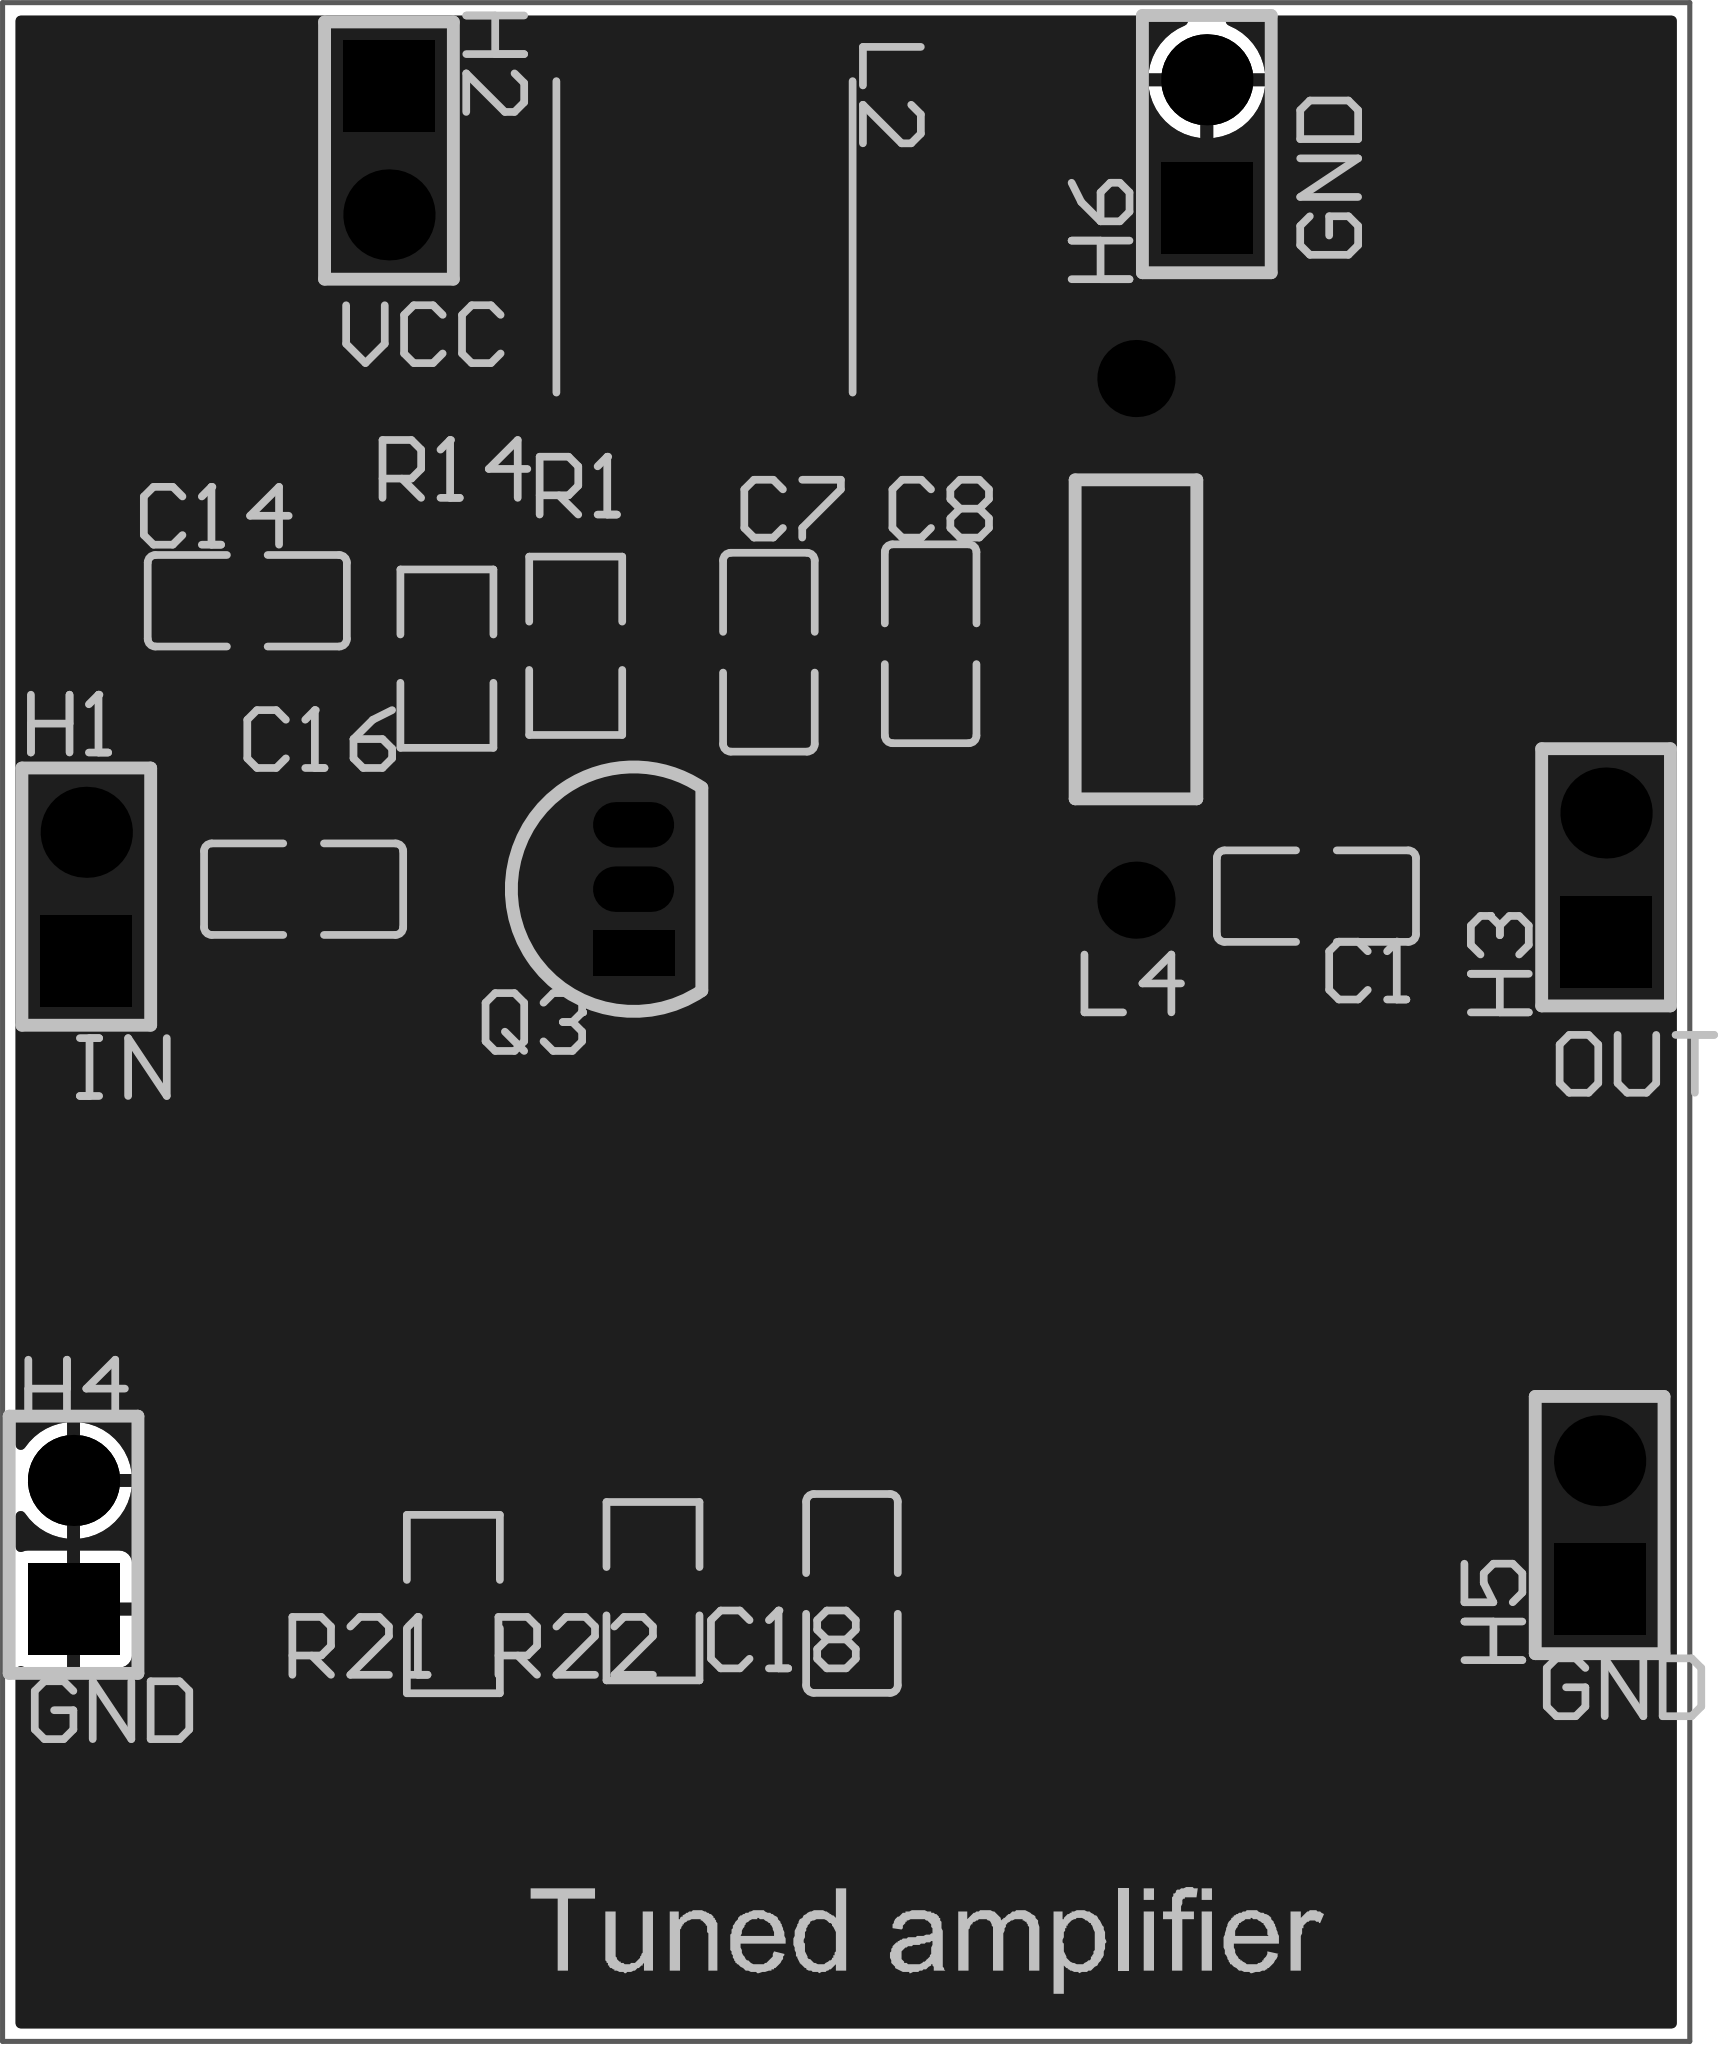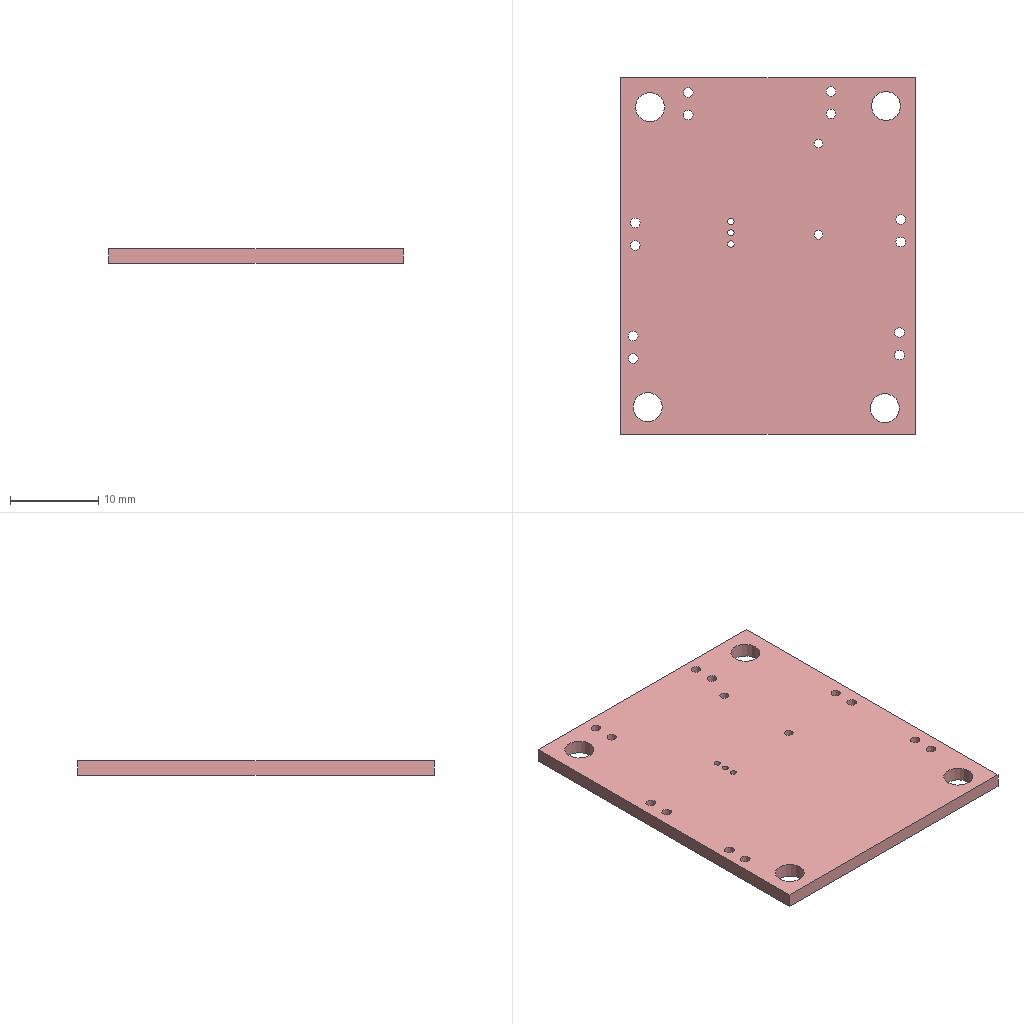Circuit board layout | Altium Designer | box 33.3 x 40.3 x 1.6 mm
Layer stack:
# Altium Designer layer stack of  (unit mm; dielectric type: 0 none, 1 core, 2 prepreg, 3 surface material)
index,name,kind,layer,copper_thickness_mm,dielectric_type,dielectric_thickness_mm,dielectric_material,dielectric_constant
0,Top Paste Mask Layer,other,,,,,,
1,Top Silkscreen Layer,other,,,,,,
2,Top Solder Mask Layer,dielectric,,,3,0.01,,3.3
3,Top Layer,copper,Top Layer,0.035,,,,
4,Dielectric1,dielectric,,,3,1.51,FR4,4.5
5,Bottom Layer,copper,Bottom Layer,0.035,,,,
6,Bottom Solder Mask Layer,dielectric,,,3,0.01,,3.3
7,Bottom Silkscreen Layer,other,,,,,,
8,Bottom Paste Mask Layer,other,,,,,,
# drill layer pairs: low layer,high layer
drill_pair,Top Layer,Bottom Layer
Part placement:
Designator,Comment,Layer,Footprint,Center-X(mm),Center-Y(mm),Rotation
C1,100nF,TopLayer,C0805,107.191,104.657,0
C7,20pF,TopLayer,C0805,96.393,109.474,90
C8,20pF,TopLayer,C0805,99.583,109.641,90
C14,100nF,TopLayer,C0805,86.106,110.49,0
C16,100nF,TopLayer,C0805,87.217,104.795,180
C18,100nF,TopLayer,C0805,98.031,90.888,270
H1,,TopLayer,HDR-TH_2P-P2.54-V-M-1,82.931,104.648,90
H2,,TopLayer,HDR-TH_2P-P2.54-V-M-1,88.9,119.38,270
H3,,TopLayer,HDR-TH_2P-P2.54-V-M-1,112.903,105.029,90
H4,,TopLayer,HDR-TH_2P-P2.54-V-M-1,82.68,91.849,90
H5,,TopLayer,HDR-TH_2P-P2.54-V-M-1,112.776,92.238,90
H6,,TopLayer,HDR-TH_2P-P2.54-V-M-1,105.029,119.507,90
L2,100uH,TopLayer,IND-SMD_L5.8-W5.2,95.123,117.602,270
L4,10kΩ,TopLayer,Res_1/4W,103.632,109.728,90
Q3,,TopLayer,S8050_TO_92,93.724,104.795,90
R1,2k,TopLayer,R0805,92.583,109.601,90
R14,15k,TopLayer,R0805,90.043,109.347,90
R21,6.2k,TopLayer,R0805,90.17,90.678,90
R22,1k,TopLayer,R0805,94.107,90.932,90
Pad and via stacks:
# Altium Designer via and pad stacks of  (unit mm). Each distinct definition once, with the count of objects using it.
# via: kind,start_layer,end_layer,hole_mm,diameter_mm,mode(0 simple;1 top-mid-bottom;2 full stack),diameter_per_layer,count,example_net
# pad: kind,layer,hole_mm,hole_type(0 round;1 square;2 slot),plating,top_size,top_shape(1 round;2 rect;3 octagon;9 rounded rect),mid_size,bottom_size,mode,footprint,size_per_layer,count,example
pad,Top Layer,0,0,plated,1.41x1.35,2,1.41x1.35,1.41x1.35,0,C0805,,12,C1.2
pad,Top Layer,0,0,plated,3x5.5,2,3x5.5,3x5.5,0,IND-SMD_L5.8-W5.2,,2,L2.1
pad,Top Layer,0,0,plated,1.133x1.377,2,1.133x1.377,1.133x1.377,0,R0805,,8,R1.2
pad,Multi-Layer,1.1,0,plated,1.8x1.8,1,1.8x1.8,1.8x1.8,0,HDR-TH_2P-P2.54-V-M-1,,6,H1.2
pad,Multi-Layer,1.1,0,plated,1.8x1.8,2,1.8x1.8,1.8x1.8,0,HDR-TH_2P-P2.54-V-M-1,,6,H1.1
pad,Multi-Layer,1,0,plated,1.524x1.524,1,1.524x1.524,1.524x1.524,0,Res_1/4W,,2,L4.1
pad,Multi-Layer,0.701,0,plated,0.8992x1.6,2,0.8992x1.6,0.8992x1.6,0,S8050_TO_92,,1,Q3.1
pad,Multi-Layer,0.701,0,plated,0.8992x1.6,1,0.8992x1.6,0.8992x1.6,0,S8050_TO_92,,2,Q3.2
Copper pours:
name,layer,net,type(0 solid;1 hatched;2 none)
Top Layer-GND,Top Layer,GND,0
Bottom Layer-GND,Bottom Layer,GND,0
Design rules, without the lines most boards share:
# Altium Designer design rules of  (exported by Altium Designer, unit mm)
# columns: name | kind | enabled | priority | scope1 | scope2 | descriptor | typed fields (field=value)
creepage | 65 | enabled | 1 | All | All | Creepage Distance Constraint =(0mil) (All),(All) |